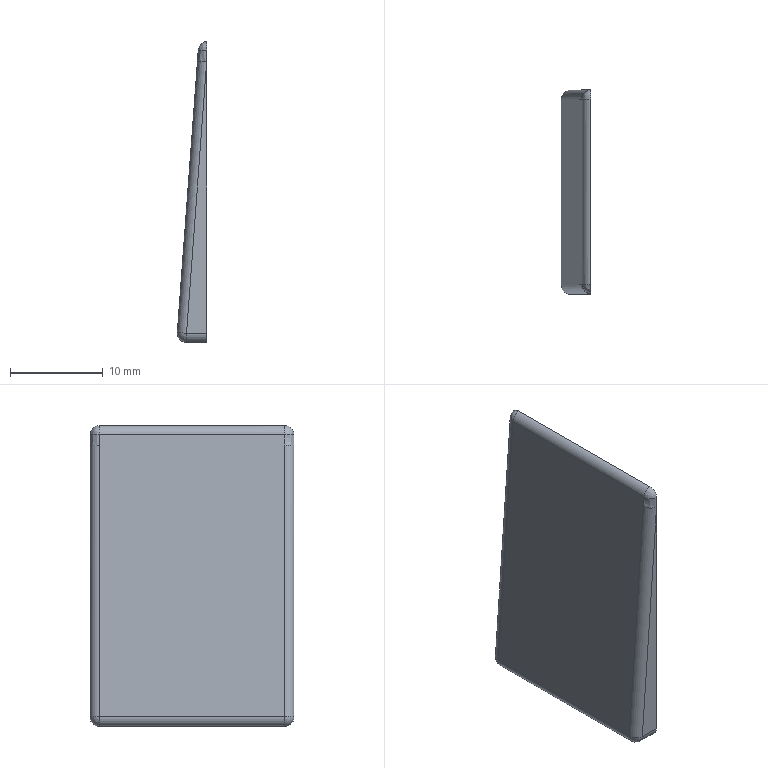Part | STEP file | Upper_shell_sub | 1 solid | 17 faces | box 3.182 x 22 x 32.446 mm | volume 1438 mm3 | cylinder 6 | plane 5 | spline 4 | sphere 2 | commonest cylinder face diameters 2 x6